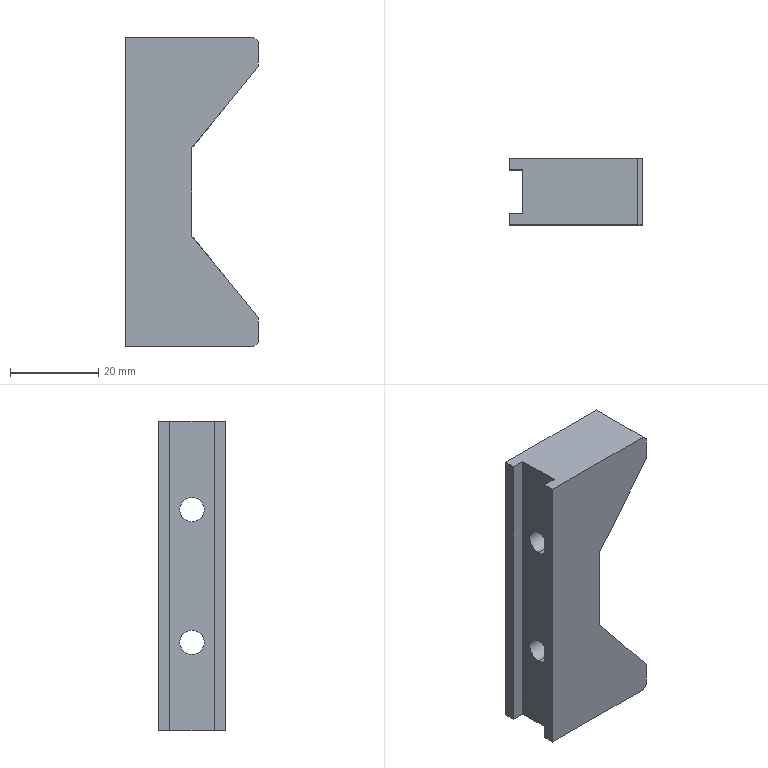Part | STEP file | 227H056247 JIG_Default | 1 solid | 26 faces | box 30 x 15 x 70 mm | volume 19012 mm3 | plane 18 | cylinder 8 | commonest cylinder face diameters 5.5 x4 9.5 x4